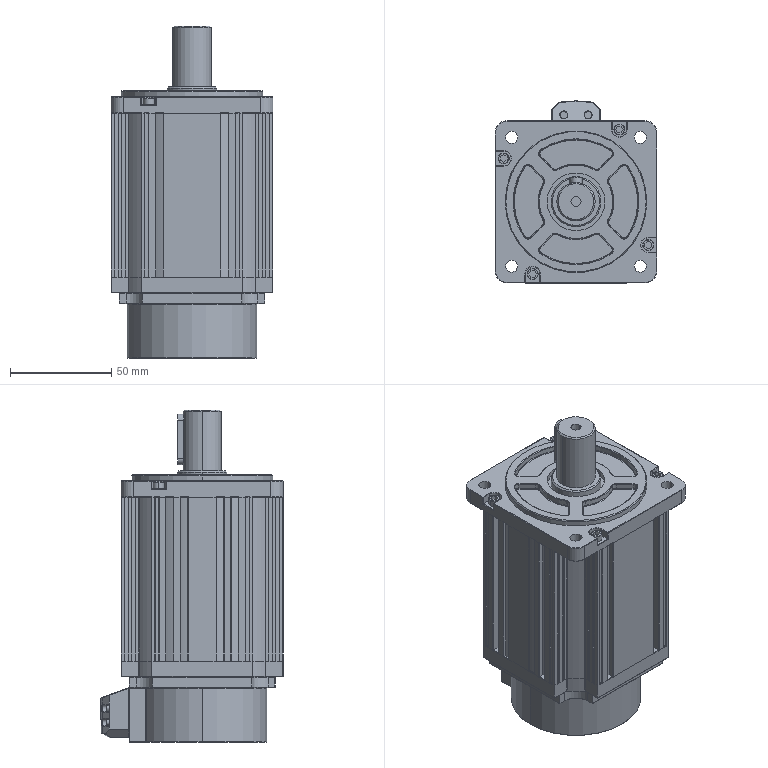Part | SolidWorks | features MBimport 1 | 1 solid | 978 faces | box 80 x 90 x 164 mm | volume 671541 mm3 | plane 394 | cylinder 364 | torus 137 | sphere 52 | spline 24 | cone 7 | commonest cylinder face diameters 0.4 x216 4.2 x20 80 x20 0.6 x16 6 x11 2.58 x8